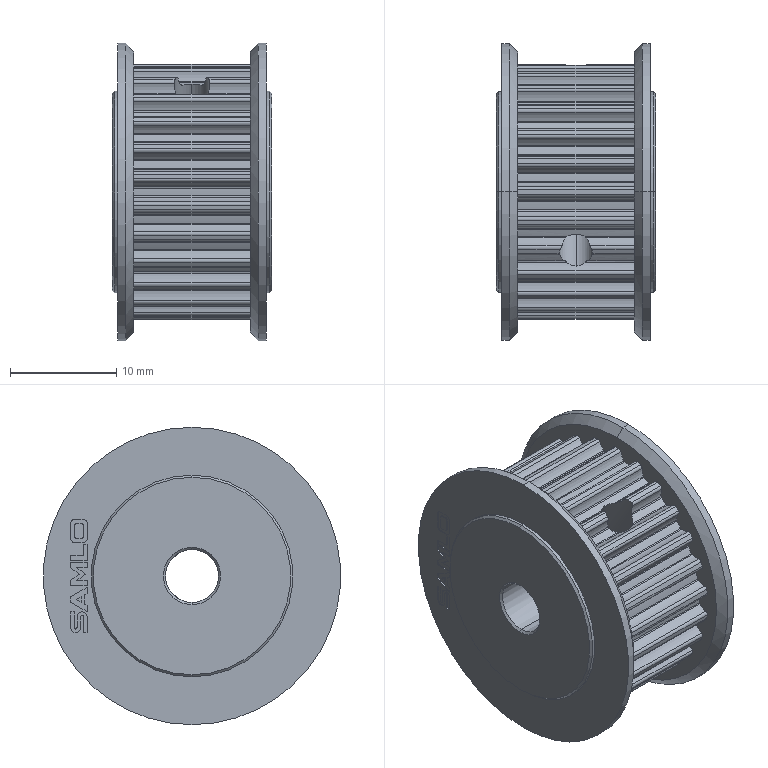Part | STEP file | TAAS3M-26-100-P5 | 1 solid | 320 faces | box 15 x 28 x 28 mm | volume 6135 mm3 | cylinder 250 | plane 58 | cone 12 | commonest cylinder face diameters 0.3 x57 0.56 x56 3.95 x56 21.85 x28 24.07 x27 0.362 x4